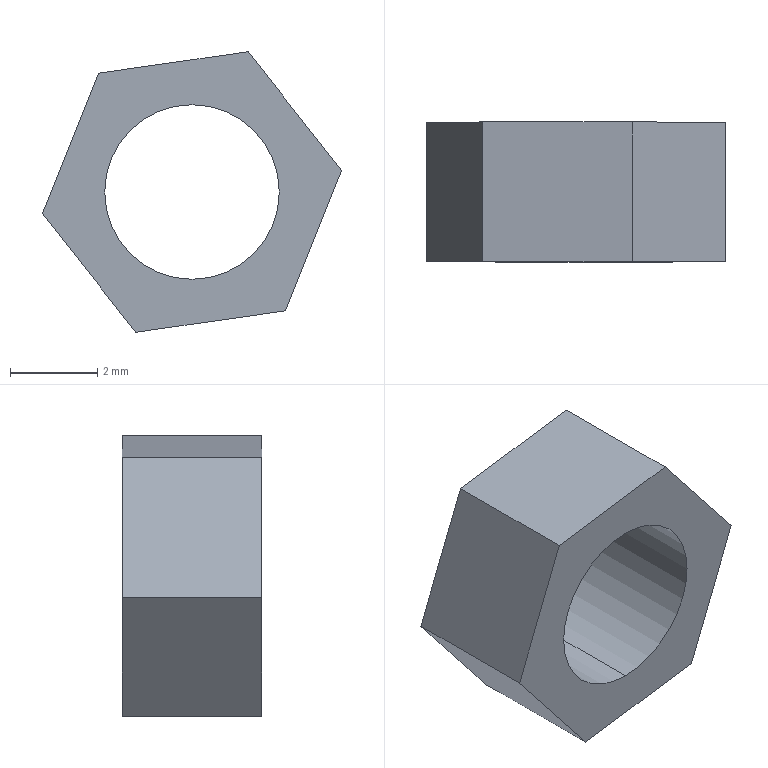Part | SolidWorks | features Extrusion 1 | 1 solid | 10 faces | box 6.858 x 3.2 x 6.431 mm | volume 59.554 mm3 | plane 8 | cylinder 2 | commonest cylinder face diameters 4 x2
STEP:
#1=CARTESIAN_POINT('',(0.,3.2,-2.));
#2=VERTEX_POINT('',#1);
#3=CARTESIAN_POINT('',(0.,3.2,2.));
#4=VERTEX_POINT('',#3);
#5=CARTESIAN_POINT('',(0.,3.2,0.));
#6=DIRECTION('',(0.,1.,0.));
#7=DIRECTION('',(0.,0.,1.));
#8=AXIS2_PLACEMENT_3D('',#5,#6,#7);
#9=CIRCLE('',#8,2.);
#10=EDGE_CURVE('',#2,#4,#9,.T.);
#11=ORIENTED_EDGE('',*,*,#10,.T.);
#12=CARTESIAN_POINT('',(0.,0.,2.));
#13=VERTEX_POINT('',#12);
#14=CARTESIAN_POINT('',(0.,3.2,2.));
#15=DIRECTION('',(0.,-1.,0.));
#16=VECTOR('',#15,1000.);
#17=LINE('',#14,#16);
#18=EDGE_CURVE('',#4,#13,#17,.T.);
#19=ORIENTED_EDGE('',*,*,#18,.T.);
#20=CARTESIAN_POINT('',(0.,0.,-2.));
#21=VERTEX_POINT('',#20);
#22=CARTESIAN_POINT('',(0.,0.,0.));
#23=DIRECTION('',(0.,1.,0.));
#24=DIRECTION('',(0.,0.,1.));
#25=AXIS2_PLACEMENT_3D('',#22,#23,#24);
#26=CIRCLE('',#25,2.);
#27=EDGE_CURVE('',#21,#13,#26,.T.);
#28=ORIENTED_EDGE('',*,*,#27,.F.);
#29=CARTESIAN_POINT('',(0.,3.2,-2.));
#30=DIRECTION('',(0.,-1.,0.));
#31=VECTOR('',#30,1000.);
#32=LINE('',#29,#31);
#33=EDGE_CURVE('',#2,#21,#32,.T.);
#34=ORIENTED_EDGE('',*,*,#33,.F.);
#35=EDGE_LOOP('',(#11,#19,#28,#34));
#36=FACE_OUTER_BOUND('',#35,.T.);
#37=CARTESIAN_POINT('',(0.,3.2,0.));
#38=DIRECTION('',(0.,-1.,0.));
#39=DIRECTION('',(0.,0.,-1.));
#40=AXIS2_PLACEMENT_3D('',#37,#38,#39);
#41=CYLINDRICAL_SURFACE('',#40,2.);
#42=ADVANCED_FACE('',(#36),#41,.F.);
#43=CARTESIAN_POINT('',(3.429,3.2,0.4924));
#44=VERTEX_POINT('',#43);
#45=CARTESIAN_POINT('',(2.141,3.2,-2.723));
#46=VERTEX_POINT('',#45);
#47=CARTESIAN_POINT('',(3.429,3.2,0.4924));
#48=DIRECTION('',(-0.3718,0.,-0.9283));
#49=VECTOR('',#48,1000.);
#50=LINE('',#47,#49);
#51=EDGE_CURVE('',#44,#46,#50,.T.);
#52=ORIENTED_EDGE('',*,*,#51,.T.);
#53=CARTESIAN_POINT('',(-1.288,3.2,-3.216));
#54=VERTEX_POINT('',#53);
#55=CARTESIAN_POINT('',(2.141,3.2,-2.723));
#56=DIRECTION('',(-0.9898,0.,-0.1421));
#57=VECTOR('',#56,1000.);
#58=LINE('',#55,#57);
#59=EDGE_CURVE('',#46,#54,#58,.T.);
#60=ORIENTED_EDGE('',*,*,#59,.T.);
#61=CARTESIAN_POINT('',(-3.429,3.2,-0.4924));
#62=VERTEX_POINT('',#61);
#63=CARTESIAN_POINT('',(-1.288,3.2,-3.216));
#64=DIRECTION('',(-0.618,0.,0.7862));
#65=VECTOR('',#64,1000.);
#66=LINE('',#63,#65);
#67=EDGE_CURVE('',#54,#62,#66,.T.);
#68=ORIENTED_EDGE('',*,*,#67,.T.);
#69=CARTESIAN_POINT('',(-2.141,3.2,2.723));
#70=VERTEX_POINT('',#69);
#71=CARTESIAN_POINT('',(-3.429,3.2,-0.4924));
#72=DIRECTION('',(0.3718,0.,0.9283));
#73=VECTOR('',#72,1000.);
#74=LINE('',#71,#73);
#75=EDGE_CURVE('',#62,#70,#74,.T.);
#76=ORIENTED_EDGE('',*,*,#75,.T.);
#77=CARTESIAN_POINT('',(1.288,3.2,3.216));
#78=VERTEX_POINT('',#77);
#79=CARTESIAN_POINT('',(-2.141,3.2,2.723));
#80=DIRECTION('',(0.9898,0.,0.1421));
#81=VECTOR('',#80,1000.);
#82=LINE('',#79,#81);
#83=EDGE_CURVE('',#70,#78,#82,.T.);
#84=ORIENTED_EDGE('',*,*,#83,.T.);
#85=CARTESIAN_POINT('',(1.288,3.2,3.216));
#86=DIRECTION('',(0.618,0.,-0.7862));
#87=VECTOR('',#86,1000.);
#88=LINE('',#85,#87);
#89=EDGE_CURVE('',#78,#44,#88,.T.);
#90=ORIENTED_EDGE('',*,*,#89,.T.);
#91=EDGE_LOOP('',(#52,#60,#68,#76,#84,#90));
#92=FACE_OUTER_BOUND('',#91,.T.);
#93=ORIENTED_EDGE('',*,*,#10,.F.);
#94=CARTESIAN_POINT('',(0.,3.2,0.));
#95=DIRECTION('',(0.,1.,0.));
#96=DIRECTION('',(0.,0.,1.));
#97=AXIS2_PLACEMENT_3D('',#94,#95,#96);
#98=CIRCLE('',#97,2.);
#99=EDGE_CURVE('',#4,#2,#98,.T.);
#100=ORIENTED_EDGE('',*,*,#99,.F.);
#101=EDGE_LOOP('',(#93,#100));
#102=FACE_BOUND('',#101,.T.);
#103=CARTESIAN_POINT('',(0.,3.2,0.));
#104=DIRECTION('',(0.,1.,0.));
#105=DIRECTION('',(0.,0.,1.));
#106=AXIS2_PLACEMENT_3D('',#103,#104,#105);
#107=PLANE('',#106);
#108=ADVANCED_FACE('',(#92,#102),#107,.T.);
#109=CARTESIAN_POINT('',(3.429,0.,0.4924));
#110=VERTEX_POINT('',#109);
#111=CARTESIAN_POINT('',(2.141,0.,-2.723));
#112=VERTEX_POINT('',#111);
#113=CARTESIAN_POINT('',(3.429,0.,0.4924));
#114=DIRECTION('',(-0.3718,0.,-0.9283));
#115=VECTOR('',#114,1000.);
#116=LINE('',#113,#115);
#117=EDGE_CURVE('',#110,#112,#116,.T.);
#118=ORIENTED_EDGE('',*,*,#117,.F.);
#119=CARTESIAN_POINT('',(1.288,0.,3.216));
#120=VERTEX_POINT('',#119);
#121=CARTESIAN_POINT('',(1.288,0.,3.216));
#122=DIRECTION('',(0.618,0.,-0.7862));
#123=VECTOR('',#122,1000.);
#124=LINE('',#121,#123);
#125=EDGE_CURVE('',#120,#110,#124,.T.);
#126=ORIENTED_EDGE('',*,*,#125,.F.);
#127=CARTESIAN_POINT('',(-2.141,0.,2.723));
#128=VERTEX_POINT('',#127);
#129=CARTESIAN_POINT('',(-2.141,0.,2.723));
#130=DIRECTION('',(0.9898,0.,0.1421));
#131=VECTOR('',#130,1000.);
#132=LINE('',#129,#131);
#133=EDGE_CURVE('',#128,#120,#132,.T.);
#134=ORIENTED_EDGE('',*,*,#133,.F.);
#135=CARTESIAN_POINT('',(-3.429,0.,-0.4924));
#136=VERTEX_POINT('',#135);
#137=CARTESIAN_POINT('',(-3.429,0.,-0.4924));
#138=DIRECTION('',(0.3718,0.,0.9283));
#139=VECTOR('',#138,1000.);
#140=LINE('',#137,#139);
#141=EDGE_CURVE('',#136,#128,#140,.T.);
#142=ORIENTED_EDGE('',*,*,#141,.F.);
#143=CARTESIAN_POINT('',(-1.288,0.,-3.216));
#144=VERTEX_POINT('',#143);
#145=CARTESIAN_POINT('',(-1.288,0.,-3.216));
#146=DIRECTION('',(-0.618,0.,0.7862));
#147=VECTOR('',#146,1000.);
#148=LINE('',#145,#147);
#149=EDGE_CURVE('',#144,#136,#148,.T.);
#150=ORIENTED_EDGE('',*,*,#149,.F.);
#151=CARTESIAN_POINT('',(2.141,0.,-2.723));
#152=DIRECTION('',(-0.9898,0.,-0.1421));
#153=VECTOR('',#152,1000.);
#154=LINE('',#151,#153);
#155=EDGE_CURVE('',#112,#144,#154,.T.);
#156=ORIENTED_EDGE('',*,*,#155,.F.);
#157=EDGE_LOOP('',(#118,#126,#134,#142,#150,#156));
#158=FACE_OUTER_BOUND('',#157,.T.);
#159=ORIENTED_EDGE('',*,*,#27,.T.);
#160=CARTESIAN_POINT('',(0.,0.,0.));
#161=DIRECTION('',(0.,1.,0.));
#162=DIRECTION('',(0.,0.,1.));
#163=AXIS2_PLACEMENT_3D('',#160,#161,#162);
#164=CIRCLE('',#163,2.);
#165=EDGE_CURVE('',#13,#21,#164,.T.);
#166=ORIENTED_EDGE('',*,*,#165,.T.);
#167=EDGE_LOOP('',(#159,#166));
#168=FACE_BOUND('',#167,.T.);
#169=CARTESIAN_POINT('',(0.,0.,0.));
#170=DIRECTION('',(0.,1.,0.));
#171=DIRECTION('',(0.,0.,1.));
#172=AXIS2_PLACEMENT_3D('',#169,#170,#171);
#173=PLANE('',#172);
#174=ADVANCED_FACE('',(#158,#168),#173,.F.);
#175=ORIENTED_EDGE('',*,*,#117,.T.);
#176=CARTESIAN_POINT('',(2.141,3.2,-2.723));
#177=DIRECTION('',(0.,-1.,0.));
#178=VECTOR('',#177,1000.);
#179=LINE('',#176,#178);
#180=EDGE_CURVE('',#46,#112,#179,.T.);
#181=ORIENTED_EDGE('',*,*,#180,.F.);
#182=ORIENTED_EDGE('',*,*,#51,.F.);
#183=CARTESIAN_POINT('',(3.429,3.2,0.4924));
#184=DIRECTION('',(0.,-1.,0.));
#185=VECTOR('',#184,1000.);
#186=LINE('',#183,#185);
#187=EDGE_CURVE('',#44,#110,#186,.T.);
#188=ORIENTED_EDGE('',*,*,#187,.T.);
#189=EDGE_LOOP('',(#175,#181,#182,#188));
#190=FACE_OUTER_BOUND('',#189,.T.);
#191=CARTESIAN_POINT('',(3.429,3.2,0.4924));
#192=DIRECTION('',(-0.9283,0.,0.3718));
#193=DIRECTION('',(0.3718,0.,0.9283));
#194=AXIS2_PLACEMENT_3D('',#191,#192,#193);
#195=PLANE('',#194);
#196=ADVANCED_FACE('',(#190),#195,.F.);
#197=ORIENTED_EDGE('',*,*,#155,.T.);
#198=CARTESIAN_POINT('',(-1.288,3.2,-3.216));
#199=DIRECTION('',(0.,-1.,0.));
#200=VECTOR('',#199,1000.);
#201=LINE('',#198,#200);
#202=EDGE_CURVE('',#54,#144,#201,.T.);
#203=ORIENTED_EDGE('',*,*,#202,.F.);
#204=ORIENTED_EDGE('',*,*,#59,.F.);
#205=ORIENTED_EDGE('',*,*,#180,.T.);
#206=EDGE_LOOP('',(#197,#203,#204,#205));
#207=FACE_OUTER_BOUND('',#206,.T.);
#208=CARTESIAN_POINT('',(2.141,3.2,-2.723));
#209=DIRECTION('',(-0.1421,0.,0.9898));
#210=DIRECTION('',(0.9898,0.,0.1421));
#211=AXIS2_PLACEMENT_3D('',#208,#209,#210);
#212=PLANE('',#211);
#213=ADVANCED_FACE('',(#207),#212,.F.);
#214=ORIENTED_EDGE('',*,*,#149,.T.);
#215=CARTESIAN_POINT('',(-3.429,3.2,-0.4924));
#216=DIRECTION('',(0.,-1.,0.));
#217=VECTOR('',#216,1000.);
#218=LINE('',#215,#217);
#219=EDGE_CURVE('',#62,#136,#218,.T.);
#220=ORIENTED_EDGE('',*,*,#219,.F.);
#221=ORIENTED_EDGE('',*,*,#67,.F.);
#222=ORIENTED_EDGE('',*,*,#202,.T.);
#223=EDGE_LOOP('',(#214,#220,#221,#222));
#224=FACE_OUTER_BOUND('',#223,.T.);
#225=CARTESIAN_POINT('',(-1.288,3.2,-3.216));
#226=DIRECTION('',(0.7862,0.,0.618));
#227=DIRECTION('',(0.618,0.,-0.7862));
#228=AXIS2_PLACEMENT_3D('',#225,#226,#227);
#229=PLANE('',#228);
#230=ADVANCED_FACE('',(#224),#229,.F.);
#231=ORIENTED_EDGE('',*,*,#141,.T.);
#232=CARTESIAN_POINT('',(-2.141,3.2,2.723));
#233=DIRECTION('',(0.,-1.,0.));
#234=VECTOR('',#233,1000.);
#235=LINE('',#232,#234);
#236=EDGE_CURVE('',#70,#128,#235,.T.);
#237=ORIENTED_EDGE('',*,*,#236,.F.);
#238=ORIENTED_EDGE('',*,*,#75,.F.);
#239=ORIENTED_EDGE('',*,*,#219,.T.);
#240=EDGE_LOOP('',(#231,#237,#238,#239));
#241=FACE_OUTER_BOUND('',#240,.T.);
#242=CARTESIAN_POINT('',(-3.429,3.2,-0.4924));
#243=DIRECTION('',(0.9283,0.,-0.3718));
#244=DIRECTION('',(-0.3718,0.,-0.9283));
#245=AXIS2_PLACEMENT_3D('',#242,#243,#244);
#246=PLANE('',#245);
#247=ADVANCED_FACE('',(#241),#246,.F.);
#248=ORIENTED_EDGE('',*,*,#133,.T.);
#249=CARTESIAN_POINT('',(1.288,3.2,3.216));
#250=DIRECTION('',(0.,-1.,0.));
#251=VECTOR('',#250,1000.);
#252=LINE('',#249,#251);
#253=EDGE_CURVE('',#78,#120,#252,.T.);
#254=ORIENTED_EDGE('',*,*,#253,.F.);
#255=ORIENTED_EDGE('',*,*,#83,.F.);
#256=ORIENTED_EDGE('',*,*,#236,.T.);
#257=EDGE_LOOP('',(#248,#254,#255,#256));
#258=FACE_OUTER_BOUND('',#257,.T.);
#259=CARTESIAN_POINT('',(-2.141,3.2,2.723));
#260=DIRECTION('',(0.1421,0.,-0.9898));
#261=DIRECTION('',(-0.9898,0.,-0.1421));
#262=AXIS2_PLACEMENT_3D('',#259,#260,#261);
#263=PLANE('',#262);
#264=ADVANCED_FACE('',(#258),#263,.F.);
#265=ORIENTED_EDGE('',*,*,#125,.T.);
#266=ORIENTED_EDGE('',*,*,#187,.F.);
#267=ORIENTED_EDGE('',*,*,#89,.F.);
#268=ORIENTED_EDGE('',*,*,#253,.T.);
#269=EDGE_LOOP('',(#265,#266,#267,#268));
#270=FACE_OUTER_BOUND('',#269,.T.);
#271=CARTESIAN_POINT('',(1.288,3.2,3.216));
#272=DIRECTION('',(-0.7862,0.,-0.618));
#273=DIRECTION('',(-0.618,0.,0.7862));
#274=AXIS2_PLACEMENT_3D('',#271,#272,#273);
#275=PLANE('',#274);
#276=ADVANCED_FACE('',(#270),#275,.F.);
#277=ORIENTED_EDGE('',*,*,#18,.F.);
#278=ORIENTED_EDGE('',*,*,#99,.T.);
#279=ORIENTED_EDGE('',*,*,#33,.T.);
#280=ORIENTED_EDGE('',*,*,#165,.F.);
#281=EDGE_LOOP('',(#277,#278,#279,#280));
#282=FACE_OUTER_BOUND('',#281,.T.);
#283=CARTESIAN_POINT('',(0.,3.2,0.));
#284=DIRECTION('',(0.,-1.,0.));
#285=DIRECTION('',(0.,0.,-1.));
#286=AXIS2_PLACEMENT_3D('',#283,#284,#285);
#287=CYLINDRICAL_SURFACE('',#286,2.);
#288=ADVANCED_FACE('',(#282),#287,.F.);
#289=CLOSED_SHELL('',(#42,#108,#174,#196,#213,#230,#247,#264,#276,#288));
#290=MANIFOLD_SOLID_BREP('',#289);
#291=CARTESIAN_POINT('',(0.,0.,0.));
#292=DIRECTION('',(0.,0.,1.));
#293=DIRECTION('',(1.,0.,0.));
#294=AXIS2_PLACEMENT_3D('',#291,#292,#293);
#295=(LENGTH_UNIT()NAMED_UNIT(*)SI_UNIT(.MILLI.,.METRE.));
#296=UNCERTAINTY_MEASURE_WITH_UNIT(LENGTH_MEASURE(0.00001),#295,'','');
#297=(NAMED_UNIT(*)PLANE_ANGLE_UNIT()SI_UNIT($,.RADIAN.));
#298=(NAMED_UNIT(*)SI_UNIT($,.STERADIAN.)SOLID_ANGLE_UNIT());
#299=(GEOMETRIC_REPRESENTATION_CONTEXT(3)GLOBAL_UNCERTAINTY_ASSIGNED_CONTEXT((#296))GLOBAL_UNIT_ASSIGNED_CONTEXT((#295,#297,#298))REPRESENTATION_CONTEXT('',''));
#300=ADVANCED_BREP_SHAPE_REPRESENTATION('',(#290,#294),#299);